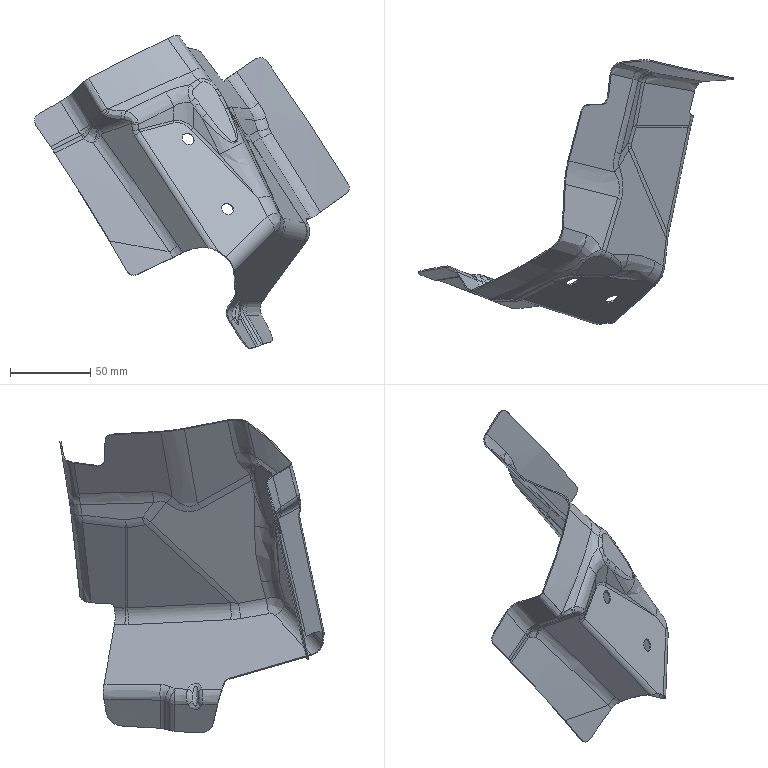Part | STEP file | FNA5401773 | 1 solid | 272 faces | box 196.776 x 165.218 x 196.033 mm | volume 33509 mm3 | spline 194 | cylinder 46 | plane 23 | other 5 | sphere 4 | commonest cylinder face diameters 8 x6 40 x5 41.6 x5 18.4 x4 20 x4 8.4 x3